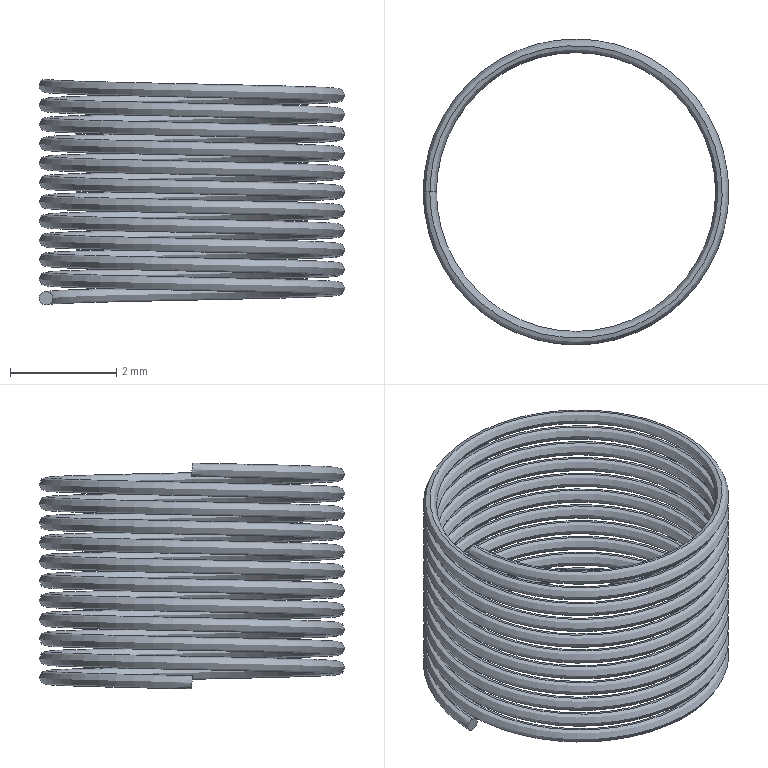Part | SolidWorks | features Helix 1, Sweep 1 | 1 solid | 4 faces | box 5.75 x 5.75 x 4.25 mm | volume 9.284 mm3 | spline 2 | plane 2